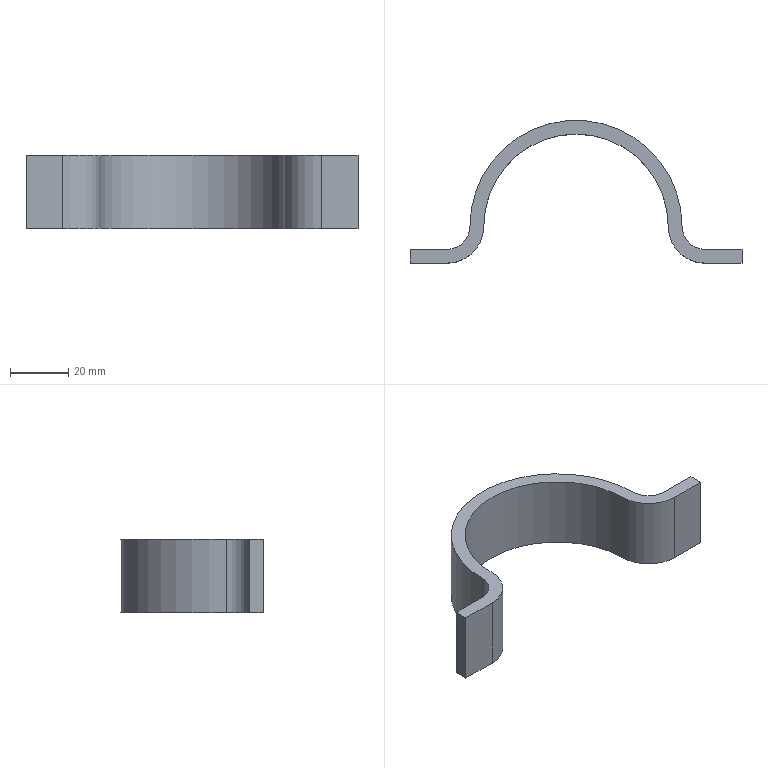Part | SolidWorks | features Extrusion 1, RefAxis 1 | 1 solid | 14 faces | box 114.3 x 49.213 x 25.4 mm | volume 19965 mm3 | plane 8 | cylinder 6 | commonest cylinder face diameters 15.875 x2 25.4 x2 63.5 x1 73.025 x1
STEP:
#1=CARTESIAN_POINT('',(-1.75,0.,-0.5));
#2=VERTEX_POINT('',#1);
#3=CARTESIAN_POINT('',(-1.25,0.5,-0.5));
#4=VERTEX_POINT('',#3);
#5=CARTESIAN_POINT('',(-1.75,0.5,-0.5));
#6=DIRECTION('',(0.,0.,1.));
#7=DIRECTION('',(1.,0.,0.));
#8=AXIS2_PLACEMENT_3D('',#5,#6,#7);
#9=CIRCLE('',#8,0.5);
#10=EDGE_CURVE('',#2,#4,#9,.T.);
#11=ORIENTED_EDGE('',*,*,#10,.T.);
#12=CARTESIAN_POINT('',(-1.25,0.5,0.5));
#13=VERTEX_POINT('',#12);
#14=CARTESIAN_POINT('',(-1.25,0.5,0.5));
#15=DIRECTION('',(0.,0.,-1.));
#16=VECTOR('',#15,39.37);
#17=LINE('',#14,#16);
#18=EDGE_CURVE('',#13,#4,#17,.T.);
#19=ORIENTED_EDGE('',*,*,#18,.F.);
#20=CARTESIAN_POINT('',(-1.75,0.,0.5));
#21=VERTEX_POINT('',#20);
#22=CARTESIAN_POINT('',(-1.75,0.5,0.5));
#23=DIRECTION('',(0.,0.,1.));
#24=DIRECTION('',(1.,0.,0.));
#25=AXIS2_PLACEMENT_3D('',#22,#23,#24);
#26=CIRCLE('',#25,0.5);
#27=EDGE_CURVE('',#21,#13,#26,.T.);
#28=ORIENTED_EDGE('',*,*,#27,.F.);
#29=CARTESIAN_POINT('',(-1.75,0.,0.5));
#30=DIRECTION('',(0.,0.,-1.));
#31=VECTOR('',#30,39.37);
#32=LINE('',#29,#31);
#33=EDGE_CURVE('',#21,#2,#32,.T.);
#34=ORIENTED_EDGE('',*,*,#33,.T.);
#35=EDGE_LOOP('',(#11,#19,#28,#34));
#36=FACE_OUTER_BOUND('',#35,.T.);
#37=CARTESIAN_POINT('',(-1.75,0.5,0.5));
#38=DIRECTION('',(0.,0.,-1.));
#39=DIRECTION('',(-1.,0.,0.));
#40=AXIS2_PLACEMENT_3D('',#37,#38,#39);
#41=CYLINDRICAL_SURFACE('',#40,0.5);
#42=ADVANCED_FACE('',(#36),#41,.T.);
#43=CARTESIAN_POINT('',(1.25,0.5,-0.5));
#44=VERTEX_POINT('',#43);
#45=CARTESIAN_POINT('',(0.,0.5,-0.5));
#46=DIRECTION('',(0.,0.,-1.));
#47=DIRECTION('',(1.,0.,0.));
#48=AXIS2_PLACEMENT_3D('',#45,#46,#47);
#49=CIRCLE('',#48,1.25);
#50=EDGE_CURVE('',#4,#44,#49,.T.);
#51=ORIENTED_EDGE('',*,*,#50,.T.);
#52=CARTESIAN_POINT('',(1.25,0.5,0.5));
#53=VERTEX_POINT('',#52);
#54=CARTESIAN_POINT('',(1.25,0.5,0.5));
#55=DIRECTION('',(0.,0.,-1.));
#56=VECTOR('',#55,39.37);
#57=LINE('',#54,#56);
#58=EDGE_CURVE('',#53,#44,#57,.T.);
#59=ORIENTED_EDGE('',*,*,#58,.F.);
#60=CARTESIAN_POINT('',(0.,0.5,0.5));
#61=DIRECTION('',(0.,0.,-1.));
#62=DIRECTION('',(1.,0.,0.));
#63=AXIS2_PLACEMENT_3D('',#60,#61,#62);
#64=CIRCLE('',#63,1.25);
#65=EDGE_CURVE('',#13,#53,#64,.T.);
#66=ORIENTED_EDGE('',*,*,#65,.F.);
#67=ORIENTED_EDGE('',*,*,#18,.T.);
#68=EDGE_LOOP('',(#51,#59,#66,#67));
#69=FACE_OUTER_BOUND('',#68,.T.);
#70=CARTESIAN_POINT('',(0.,0.5,0.5));
#71=DIRECTION('',(0.,0.,-1.));
#72=DIRECTION('',(-1.,0.,0.));
#73=AXIS2_PLACEMENT_3D('',#70,#71,#72);
#74=CYLINDRICAL_SURFACE('',#73,1.25);
#75=ADVANCED_FACE('',(#69),#74,.F.);
#76=CARTESIAN_POINT('',(1.75,0.,-0.5));
#77=VERTEX_POINT('',#76);
#78=CARTESIAN_POINT('',(1.75,0.5,-0.5));
#79=DIRECTION('',(0.,0.,1.));
#80=DIRECTION('',(-1.,0.,0.));
#81=AXIS2_PLACEMENT_3D('',#78,#79,#80);
#82=CIRCLE('',#81,0.5);
#83=EDGE_CURVE('',#44,#77,#82,.T.);
#84=ORIENTED_EDGE('',*,*,#83,.T.);
#85=CARTESIAN_POINT('',(1.75,0.,0.5));
#86=VERTEX_POINT('',#85);
#87=CARTESIAN_POINT('',(1.75,0.,0.5));
#88=DIRECTION('',(0.,0.,-1.));
#89=VECTOR('',#88,39.37);
#90=LINE('',#87,#89);
#91=EDGE_CURVE('',#86,#77,#90,.T.);
#92=ORIENTED_EDGE('',*,*,#91,.F.);
#93=CARTESIAN_POINT('',(1.75,0.5,0.5));
#94=DIRECTION('',(0.,0.,1.));
#95=DIRECTION('',(-1.,0.,0.));
#96=AXIS2_PLACEMENT_3D('',#93,#94,#95);
#97=CIRCLE('',#96,0.5);
#98=EDGE_CURVE('',#53,#86,#97,.T.);
#99=ORIENTED_EDGE('',*,*,#98,.F.);
#100=ORIENTED_EDGE('',*,*,#58,.T.);
#101=EDGE_LOOP('',(#84,#92,#99,#100));
#102=FACE_OUTER_BOUND('',#101,.T.);
#103=CARTESIAN_POINT('',(1.75,0.5,0.5));
#104=DIRECTION('',(0.,0.,-1.));
#105=DIRECTION('',(-1.,0.,0.));
#106=AXIS2_PLACEMENT_3D('',#103,#104,#105);
#107=CYLINDRICAL_SURFACE('',#106,0.5);
#108=ADVANCED_FACE('',(#102),#107,.T.);
#109=CARTESIAN_POINT('',(2.25,0.,-0.5));
#110=VERTEX_POINT('',#109);
#111=CARTESIAN_POINT('',(1.75,0.,-0.5));
#112=DIRECTION('',(1.,0.,0.));
#113=VECTOR('',#112,39.37);
#114=LINE('',#111,#113);
#115=EDGE_CURVE('',#77,#110,#114,.T.);
#116=ORIENTED_EDGE('',*,*,#115,.T.);
#117=CARTESIAN_POINT('',(2.25,0.,0.5));
#118=VERTEX_POINT('',#117);
#119=CARTESIAN_POINT('',(2.25,0.,0.5));
#120=DIRECTION('',(0.,0.,-1.));
#121=VECTOR('',#120,39.37);
#122=LINE('',#119,#121);
#123=EDGE_CURVE('',#118,#110,#122,.T.);
#124=ORIENTED_EDGE('',*,*,#123,.F.);
#125=CARTESIAN_POINT('',(1.75,0.,0.5));
#126=DIRECTION('',(1.,0.,0.));
#127=VECTOR('',#126,39.37);
#128=LINE('',#125,#127);
#129=EDGE_CURVE('',#86,#118,#128,.T.);
#130=ORIENTED_EDGE('',*,*,#129,.F.);
#131=ORIENTED_EDGE('',*,*,#91,.T.);
#132=EDGE_LOOP('',(#116,#124,#130,#131));
#133=FACE_OUTER_BOUND('',#132,.T.);
#134=CARTESIAN_POINT('',(1.75,0.,0.5));
#135=DIRECTION('',(0.,1.,0.));
#136=DIRECTION('',(-1.,0.,0.));
#137=AXIS2_PLACEMENT_3D('',#134,#135,#136);
#138=PLANE('',#137);
#139=ADVANCED_FACE('',(#133),#138,.F.);
#140=CARTESIAN_POINT('',(2.25,0.1875,-0.5));
#141=VERTEX_POINT('',#140);
#142=CARTESIAN_POINT('',(2.25,0.,-0.5));
#143=DIRECTION('',(0.,1.,0.));
#144=VECTOR('',#143,39.37);
#145=LINE('',#142,#144);
#146=EDGE_CURVE('',#110,#141,#145,.T.);
#147=ORIENTED_EDGE('',*,*,#146,.T.);
#148=CARTESIAN_POINT('',(2.25,0.1875,0.5));
#149=VERTEX_POINT('',#148);
#150=CARTESIAN_POINT('',(2.25,0.1875,0.5));
#151=DIRECTION('',(0.,0.,-1.));
#152=VECTOR('',#151,39.37);
#153=LINE('',#150,#152);
#154=EDGE_CURVE('',#149,#141,#153,.T.);
#155=ORIENTED_EDGE('',*,*,#154,.F.);
#156=CARTESIAN_POINT('',(2.25,0.,0.5));
#157=DIRECTION('',(0.,1.,0.));
#158=VECTOR('',#157,39.37);
#159=LINE('',#156,#158);
#160=EDGE_CURVE('',#118,#149,#159,.T.);
#161=ORIENTED_EDGE('',*,*,#160,.F.);
#162=ORIENTED_EDGE('',*,*,#123,.T.);
#163=EDGE_LOOP('',(#147,#155,#161,#162));
#164=FACE_OUTER_BOUND('',#163,.T.);
#165=CARTESIAN_POINT('',(2.25,0.,0.5));
#166=DIRECTION('',(-1.,0.,0.));
#167=DIRECTION('',(0.,-1.,0.));
#168=AXIS2_PLACEMENT_3D('',#165,#166,#167);
#169=PLANE('',#168);
#170=ADVANCED_FACE('',(#164),#169,.F.);
#171=CARTESIAN_POINT('',(1.75,0.1875,-0.5));
#172=VERTEX_POINT('',#171);
#173=CARTESIAN_POINT('',(2.25,0.1875,-0.5));
#174=DIRECTION('',(-1.,0.,0.));
#175=VECTOR('',#174,39.37);
#176=LINE('',#173,#175);
#177=EDGE_CURVE('',#141,#172,#176,.T.);
#178=ORIENTED_EDGE('',*,*,#177,.T.);
#179=CARTESIAN_POINT('',(1.75,0.1875,0.5));
#180=VERTEX_POINT('',#179);
#181=CARTESIAN_POINT('',(1.75,0.1875,0.5));
#182=DIRECTION('',(0.,0.,-1.));
#183=VECTOR('',#182,39.37);
#184=LINE('',#181,#183);
#185=EDGE_CURVE('',#180,#172,#184,.T.);
#186=ORIENTED_EDGE('',*,*,#185,.F.);
#187=CARTESIAN_POINT('',(2.25,0.1875,0.5));
#188=DIRECTION('',(-1.,0.,0.));
#189=VECTOR('',#188,39.37);
#190=LINE('',#187,#189);
#191=EDGE_CURVE('',#149,#180,#190,.T.);
#192=ORIENTED_EDGE('',*,*,#191,.F.);
#193=ORIENTED_EDGE('',*,*,#154,.T.);
#194=EDGE_LOOP('',(#178,#186,#192,#193));
#195=FACE_OUTER_BOUND('',#194,.T.);
#196=CARTESIAN_POINT('',(2.25,0.1875,0.5));
#197=DIRECTION('',(0.,-1.,0.));
#198=DIRECTION('',(0.,0.,-1.));
#199=AXIS2_PLACEMENT_3D('',#196,#197,#198);
#200=PLANE('',#199);
#201=ADVANCED_FACE('',(#195),#200,.F.);
#202=CARTESIAN_POINT('',(1.438,0.5,-0.5));
#203=VERTEX_POINT('',#202);
#204=CARTESIAN_POINT('',(1.75,0.5,-0.5));
#205=DIRECTION('',(0.,0.,-1.));
#206=DIRECTION('',(-1.,0.,0.));
#207=AXIS2_PLACEMENT_3D('',#204,#205,#206);
#208=CIRCLE('',#207,0.3125);
#209=EDGE_CURVE('',#172,#203,#208,.T.);
#210=ORIENTED_EDGE('',*,*,#209,.T.);
#211=CARTESIAN_POINT('',(1.438,0.5,0.5));
#212=VERTEX_POINT('',#211);
#213=CARTESIAN_POINT('',(1.438,0.5,0.5));
#214=DIRECTION('',(0.,0.,-1.));
#215=VECTOR('',#214,39.37);
#216=LINE('',#213,#215);
#217=EDGE_CURVE('',#212,#203,#216,.T.);
#218=ORIENTED_EDGE('',*,*,#217,.F.);
#219=CARTESIAN_POINT('',(1.75,0.5,0.5));
#220=DIRECTION('',(0.,0.,-1.));
#221=DIRECTION('',(-1.,0.,0.));
#222=AXIS2_PLACEMENT_3D('',#219,#220,#221);
#223=CIRCLE('',#222,0.3125);
#224=EDGE_CURVE('',#180,#212,#223,.T.);
#225=ORIENTED_EDGE('',*,*,#224,.F.);
#226=ORIENTED_EDGE('',*,*,#185,.T.);
#227=EDGE_LOOP('',(#210,#218,#225,#226));
#228=FACE_OUTER_BOUND('',#227,.T.);
#229=CARTESIAN_POINT('',(1.75,0.5,0.5));
#230=DIRECTION('',(0.,0.,-1.));
#231=DIRECTION('',(-1.,0.,0.));
#232=AXIS2_PLACEMENT_3D('',#229,#230,#231);
#233=CYLINDRICAL_SURFACE('',#232,0.3125);
#234=ADVANCED_FACE('',(#228),#233,.F.);
#235=CARTESIAN_POINT('',(-1.438,0.5,-0.5));
#236=VERTEX_POINT('',#235);
#237=CARTESIAN_POINT('',(0.,0.5,-0.5));
#238=DIRECTION('',(0.,0.,1.));
#239=DIRECTION('',(1.,0.,0.));
#240=AXIS2_PLACEMENT_3D('',#237,#238,#239);
#241=CIRCLE('',#240,1.438);
#242=EDGE_CURVE('',#203,#236,#241,.T.);
#243=ORIENTED_EDGE('',*,*,#242,.T.);
#244=CARTESIAN_POINT('',(-1.438,0.5,0.5));
#245=VERTEX_POINT('',#244);
#246=CARTESIAN_POINT('',(-1.438,0.5,0.5));
#247=DIRECTION('',(0.,0.,-1.));
#248=VECTOR('',#247,39.37);
#249=LINE('',#246,#248);
#250=EDGE_CURVE('',#245,#236,#249,.T.);
#251=ORIENTED_EDGE('',*,*,#250,.F.);
#252=CARTESIAN_POINT('',(0.,0.5,0.5));
#253=DIRECTION('',(0.,0.,1.));
#254=DIRECTION('',(1.,0.,0.));
#255=AXIS2_PLACEMENT_3D('',#252,#253,#254);
#256=CIRCLE('',#255,1.438);
#257=EDGE_CURVE('',#212,#245,#256,.T.);
#258=ORIENTED_EDGE('',*,*,#257,.F.);
#259=ORIENTED_EDGE('',*,*,#217,.T.);
#260=EDGE_LOOP('',(#243,#251,#258,#259));
#261=FACE_OUTER_BOUND('',#260,.T.);
#262=CARTESIAN_POINT('',(0.,0.5,0.5));
#263=DIRECTION('',(0.,0.,-1.));
#264=DIRECTION('',(-1.,0.,0.));
#265=AXIS2_PLACEMENT_3D('',#262,#263,#264);
#266=CYLINDRICAL_SURFACE('',#265,1.438);
#267=ADVANCED_FACE('',(#261),#266,.T.);
#268=CARTESIAN_POINT('',(-1.75,0.1875,-0.5));
#269=VERTEX_POINT('',#268);
#270=CARTESIAN_POINT('',(-1.75,0.5,-0.5));
#271=DIRECTION('',(0.,0.,-1.));
#272=DIRECTION('',(1.,0.,0.));
#273=AXIS2_PLACEMENT_3D('',#270,#271,#272);
#274=CIRCLE('',#273,0.3125);
#275=EDGE_CURVE('',#236,#269,#274,.T.);
#276=ORIENTED_EDGE('',*,*,#275,.T.);
#277=CARTESIAN_POINT('',(-1.75,0.1875,0.5));
#278=VERTEX_POINT('',#277);
#279=CARTESIAN_POINT('',(-1.75,0.1875,0.5));
#280=DIRECTION('',(0.,0.,-1.));
#281=VECTOR('',#280,39.37);
#282=LINE('',#279,#281);
#283=EDGE_CURVE('',#278,#269,#282,.T.);
#284=ORIENTED_EDGE('',*,*,#283,.F.);
#285=CARTESIAN_POINT('',(-1.75,0.5,0.5));
#286=DIRECTION('',(0.,0.,-1.));
#287=DIRECTION('',(1.,0.,0.));
#288=AXIS2_PLACEMENT_3D('',#285,#286,#287);
#289=CIRCLE('',#288,0.3125);
#290=EDGE_CURVE('',#245,#278,#289,.T.);
#291=ORIENTED_EDGE('',*,*,#290,.F.);
#292=ORIENTED_EDGE('',*,*,#250,.T.);
#293=EDGE_LOOP('',(#276,#284,#291,#292));
#294=FACE_OUTER_BOUND('',#293,.T.);
#295=CARTESIAN_POINT('',(-1.75,0.5,0.5));
#296=DIRECTION('',(0.,0.,-1.));
#297=DIRECTION('',(-1.,0.,0.));
#298=AXIS2_PLACEMENT_3D('',#295,#296,#297);
#299=CYLINDRICAL_SURFACE('',#298,0.3125);
#300=ADVANCED_FACE('',(#294),#299,.F.);
#301=CARTESIAN_POINT('',(-2.25,0.1875,-0.5));
#302=VERTEX_POINT('',#301);
#303=CARTESIAN_POINT('',(-2.25,0.1875,-0.5));
#304=DIRECTION('',(-1.,0.,0.));
#305=VECTOR('',#304,39.37);
#306=LINE('',#303,#305);
#307=EDGE_CURVE('',#269,#302,#306,.T.);
#308=ORIENTED_EDGE('',*,*,#307,.T.);
#309=CARTESIAN_POINT('',(-2.25,0.1875,0.5));
#310=VERTEX_POINT('',#309);
#311=CARTESIAN_POINT('',(-2.25,0.1875,0.5));
#312=DIRECTION('',(0.,0.,-1.));
#313=VECTOR('',#312,39.37);
#314=LINE('',#311,#313);
#315=EDGE_CURVE('',#310,#302,#314,.T.);
#316=ORIENTED_EDGE('',*,*,#315,.F.);
#317=CARTESIAN_POINT('',(-2.25,0.1875,0.5));
#318=DIRECTION('',(-1.,0.,0.));
#319=VECTOR('',#318,39.37);
#320=LINE('',#317,#319);
#321=EDGE_CURVE('',#278,#310,#320,.T.);
#322=ORIENTED_EDGE('',*,*,#321,.F.);
#323=ORIENTED_EDGE('',*,*,#283,.T.);
#324=EDGE_LOOP('',(#308,#316,#322,#323));
#325=FACE_OUTER_BOUND('',#324,.T.);
#326=CARTESIAN_POINT('',(-2.25,0.1875,0.5));
#327=DIRECTION('',(0.,-1.,0.));
#328=DIRECTION('',(0.,0.,-1.));
#329=AXIS2_PLACEMENT_3D('',#326,#327,#328);
#330=PLANE('',#329);
#331=ADVANCED_FACE('',(#325),#330,.F.);
#332=CARTESIAN_POINT('',(-2.25,0.,-0.5));
#333=VERTEX_POINT('',#332);
#334=CARTESIAN_POINT('',(-2.25,0.,-0.5));
#335=DIRECTION('',(0.,-1.,0.));
#336=VECTOR('',#335,39.37);
#337=LINE('',#334,#336);
#338=EDGE_CURVE('',#302,#333,#337,.T.);
#339=ORIENTED_EDGE('',*,*,#338,.T.);
#340=CARTESIAN_POINT('',(-2.25,0.,0.5));
#341=VERTEX_POINT('',#340);
#342=CARTESIAN_POINT('',(-2.25,0.,0.5));
#343=DIRECTION('',(0.,0.,-1.));
#344=VECTOR('',#343,39.37);
#345=LINE('',#342,#344);
#346=EDGE_CURVE('',#341,#333,#345,.T.);
#347=ORIENTED_EDGE('',*,*,#346,.F.);
#348=CARTESIAN_POINT('',(-2.25,0.,0.5));
#349=DIRECTION('',(0.,-1.,0.));
#350=VECTOR('',#349,39.37);
#351=LINE('',#348,#350);
#352=EDGE_CURVE('',#310,#341,#351,.T.);
#353=ORIENTED_EDGE('',*,*,#352,.F.);
#354=ORIENTED_EDGE('',*,*,#315,.T.);
#355=EDGE_LOOP('',(#339,#347,#353,#354));
#356=FACE_OUTER_BOUND('',#355,.T.);
#357=CARTESIAN_POINT('',(-2.25,0.,0.5));
#358=DIRECTION('',(1.,0.,0.));
#359=DIRECTION('',(0.,1.,0.));
#360=AXIS2_PLACEMENT_3D('',#357,#358,#359);
#361=PLANE('',#360);
#362=ADVANCED_FACE('',(#356),#361,.F.);
#363=CARTESIAN_POINT('',(-1.75,0.,-0.5));
#364=DIRECTION('',(1.,0.,0.));
#365=VECTOR('',#364,39.37);
#366=LINE('',#363,#365);
#367=EDGE_CURVE('',#333,#2,#366,.T.);
#368=ORIENTED_EDGE('',*,*,#367,.T.);
#369=ORIENTED_EDGE('',*,*,#33,.F.);
#370=CARTESIAN_POINT('',(-1.75,0.,0.5));
#371=DIRECTION('',(1.,0.,0.));
#372=VECTOR('',#371,39.37);
#373=LINE('',#370,#372);
#374=EDGE_CURVE('',#341,#21,#373,.T.);
#375=ORIENTED_EDGE('',*,*,#374,.F.);
#376=ORIENTED_EDGE('',*,*,#346,.T.);
#377=EDGE_LOOP('',(#368,#369,#375,#376));
#378=FACE_OUTER_BOUND('',#377,.T.);
#379=CARTESIAN_POINT('',(-1.75,0.,0.5));
#380=DIRECTION('',(0.,1.,0.));
#381=DIRECTION('',(-1.,0.,0.));
#382=AXIS2_PLACEMENT_3D('',#379,#380,#381);
#383=PLANE('',#382);
#384=ADVANCED_FACE('',(#378),#383,.F.);
#385=ORIENTED_EDGE('',*,*,#27,.T.);
#386=ORIENTED_EDGE('',*,*,#65,.T.);
#387=ORIENTED_EDGE('',*,*,#98,.T.);
#388=ORIENTED_EDGE('',*,*,#129,.T.);
#389=ORIENTED_EDGE('',*,*,#160,.T.);
#390=ORIENTED_EDGE('',*,*,#191,.T.);
#391=ORIENTED_EDGE('',*,*,#224,.T.);
#392=ORIENTED_EDGE('',*,*,#257,.T.);
#393=ORIENTED_EDGE('',*,*,#290,.T.);
#394=ORIENTED_EDGE('',*,*,#321,.T.);
#395=ORIENTED_EDGE('',*,*,#352,.T.);
#396=ORIENTED_EDGE('',*,*,#374,.T.);
#397=EDGE_LOOP('',(#385,#386,#387,#388,#389,#390,#391,#392,#393,#394,#395,#396));
#398=FACE_OUTER_BOUND('',#397,.T.);
#399=CARTESIAN_POINT('',(-1.75,0.5,0.5));
#400=DIRECTION('',(0.,0.,1.));
#401=DIRECTION('',(1.,0.,0.));
#402=AXIS2_PLACEMENT_3D('',#399,#400,#401);
#403=PLANE('',#402);
#404=ADVANCED_FACE('',(#398),#403,.T.);
#405=ORIENTED_EDGE('',*,*,#10,.F.);
#406=ORIENTED_EDGE('',*,*,#367,.F.);
#407=ORIENTED_EDGE('',*,*,#338,.F.);
#408=ORIENTED_EDGE('',*,*,#307,.F.);
#409=ORIENTED_EDGE('',*,*,#275,.F.);
#410=ORIENTED_EDGE('',*,*,#242,.F.);
#411=ORIENTED_EDGE('',*,*,#209,.F.);
#412=ORIENTED_EDGE('',*,*,#177,.F.);
#413=ORIENTED_EDGE('',*,*,#146,.F.);
#414=ORIENTED_EDGE('',*,*,#115,.F.);
#415=ORIENTED_EDGE('',*,*,#83,.F.);
#416=ORIENTED_EDGE('',*,*,#50,.F.);
#417=EDGE_LOOP('',(#405,#406,#407,#408,#409,#410,#411,#412,#413,#414,#415,#416));
#418=FACE_OUTER_BOUND('',#417,.T.);
#419=CARTESIAN_POINT('',(-1.75,0.5,-0.5));
#420=DIRECTION('',(0.,0.,1.));
#421=DIRECTION('',(1.,0.,0.));
#422=AXIS2_PLACEMENT_3D('',#419,#420,#421);
#423=PLANE('',#422);
#424=ADVANCED_FACE('',(#418),#423,.F.);
#425=CLOSED_SHELL('',(#42,#75,#108,#139,#170,#201,#234,#267,#300,#331,#362,#384,#404,#424));
#426=MANIFOLD_SOLID_BREP('',#425);
#427=CARTESIAN_POINT('',(0.,0.,0.));
#428=DIRECTION('',(0.,0.,1.));
#429=DIRECTION('',(1.,0.,0.));
#430=AXIS2_PLACEMENT_3D('',#427,#428,#429);
#431=(LENGTH_UNIT()NAMED_UNIT(*)SI_UNIT($,.METRE.));
#432=LENGTH_MEASURE_WITH_UNIT(LENGTH_MEASURE(0.0254),#431);
#433=DIMENSIONAL_EXPONENTS(1.,0.,0.,0.,0.,0.,0.);
#434=(CONVERSION_BASED_UNIT('INCH',#432)LENGTH_UNIT()NAMED_UNIT(#433));
#435=UNCERTAINTY_MEASURE_WITH_UNIT(LENGTH_MEASURE(0.00001),#434,'','');
#436=(NAMED_UNIT(*)PLANE_ANGLE_UNIT()SI_UNIT($,.RADIAN.));
#437=(NAMED_UNIT(*)SI_UNIT($,.STERADIAN.)SOLID_ANGLE_UNIT());
#438=(GEOMETRIC_REPRESENTATION_CONTEXT(3)GLOBAL_UNCERTAINTY_ASSIGNED_CONTEXT((#435))GLOBAL_UNIT_ASSIGNED_CONTEXT((#434,#436,#437))REPRESENTATION_CONTEXT('',''));
#439=ADVANCED_BREP_SHAPE_REPRESENTATION('',(#426,#430),#438);